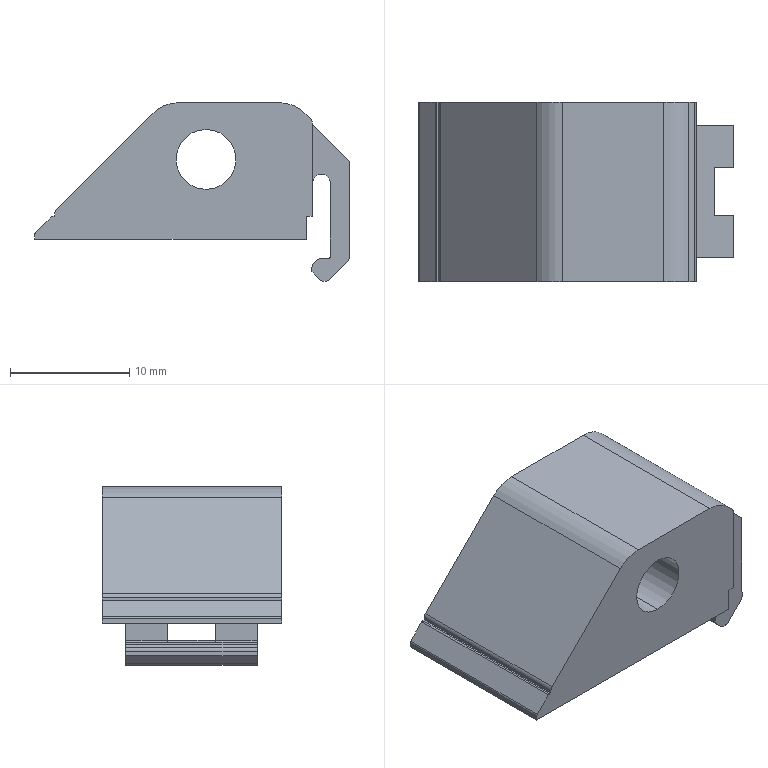Part | SolidWorks | features BaseBody 1 | 1 solid | 49 faces | box 26.35 x 15 x 14.95 mm | volume 2648 mm3 | plane 31 | cylinder 18 | commonest cylinder face diameters 1 x7 0.4 x3 5 x2 6 x2 8.2 x2 1.002 x1